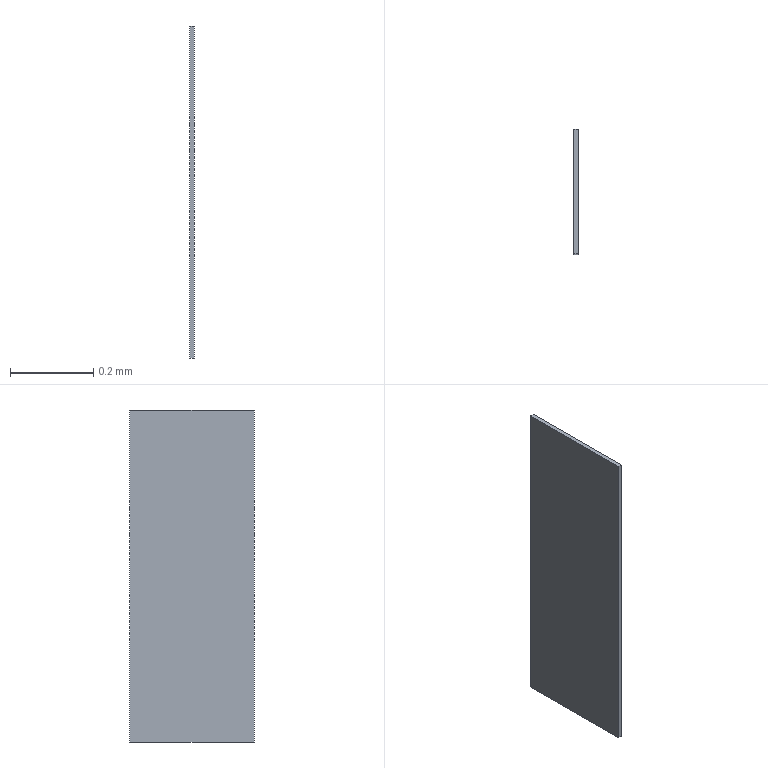Part | Creo | 1 solid | 6 faces | box 0.01 x 0.3 x 0.8 mm | volume 0.0024 mm3 | plane 6
STEP:
#1=CARTESIAN_POINT('',(0.,0.,0.));
#2=DIRECTION('',(0.,0.,1.));
#3=DIRECTION('',(1.,0.,0.));
#4=AXIS2_PLACEMENT_3D('',#1,#2,#3);
#5=CARTESIAN_POINT('',(0.12,-5.55,1.08));
#6=VERTEX_POINT('',#5);
#7=CARTESIAN_POINT('',(0.12,-5.55,1.88));
#8=VERTEX_POINT('',#7);
#9=CARTESIAN_POINT('',(0.12,-5.55,1.08));
#10=DIRECTION('',(0.,0.,1.));
#11=VECTOR('',#10,0.8);
#12=LINE('',#9,#11);
#13=EDGE_CURVE('',#6,#8,#12,.T.);
#14=ORIENTED_EDGE('',*,*,#13,.F.);
#15=CARTESIAN_POINT('',(0.12,-5.85,1.08));
#16=VERTEX_POINT('',#15);
#17=CARTESIAN_POINT('',(0.12,-5.85,1.08));
#18=DIRECTION('',(0.,1.,0.));
#19=VECTOR('',#18,0.3);
#20=LINE('',#17,#19);
#21=EDGE_CURVE('',#16,#6,#20,.T.);
#22=ORIENTED_EDGE('',*,*,#21,.F.);
#23=CARTESIAN_POINT('',(0.12,-5.85,1.88));
#24=VERTEX_POINT('',#23);
#25=CARTESIAN_POINT('',(0.12,-5.85,1.88));
#26=DIRECTION('',(0.,0.,-1.));
#27=VECTOR('',#26,0.8);
#28=LINE('',#25,#27);
#29=EDGE_CURVE('',#24,#16,#28,.T.);
#30=ORIENTED_EDGE('',*,*,#29,.F.);
#31=CARTESIAN_POINT('',(0.12,-5.55,1.88));
#32=DIRECTION('',(0.,-1.,0.));
#33=VECTOR('',#32,0.3);
#34=LINE('',#31,#33);
#35=EDGE_CURVE('',#8,#24,#34,.T.);
#36=ORIENTED_EDGE('',*,*,#35,.F.);
#37=EDGE_LOOP('',(#14,#22,#30,#36));
#38=FACE_OUTER_BOUND('',#37,.F.);
#39=CARTESIAN_POINT('',(0.12,0.,0.));
#40=DIRECTION('',(1.,0.,0.));
#41=DIRECTION('',(0.,-1.,0.));
#42=AXIS2_PLACEMENT_3D('',#39,#40,#41);
#43=PLANE('',#42);
#44=ADVANCED_FACE('',(#38),#43,.T.);
#45=CARTESIAN_POINT('',(0.11,-5.55,1.08));
#46=VERTEX_POINT('',#45);
#47=CARTESIAN_POINT('',(0.11,-5.55,1.88));
#48=VERTEX_POINT('',#47);
#49=CARTESIAN_POINT('',(0.11,-5.55,1.08));
#50=DIRECTION('',(0.,0.,1.));
#51=VECTOR('',#50,0.8);
#52=LINE('',#49,#51);
#53=EDGE_CURVE('',#46,#48,#52,.T.);
#54=ORIENTED_EDGE('',*,*,#53,.F.);
#55=CARTESIAN_POINT('',(0.11,-5.55,1.08));
#56=DIRECTION('',(1.,0.,0.));
#57=VECTOR('',#56,0.01);
#58=LINE('',#55,#57);
#59=EDGE_CURVE('',#46,#6,#58,.T.);
#60=ORIENTED_EDGE('',*,*,#59,.T.);
#61=ORIENTED_EDGE('',*,*,#13,.T.);
#62=CARTESIAN_POINT('',(0.11,-5.55,1.88));
#63=DIRECTION('',(1.,0.,0.));
#64=VECTOR('',#63,0.01);
#65=LINE('',#62,#64);
#66=EDGE_CURVE('',#48,#8,#65,.T.);
#67=ORIENTED_EDGE('',*,*,#66,.F.);
#68=EDGE_LOOP('',(#54,#60,#61,#67));
#69=FACE_OUTER_BOUND('',#68,.F.);
#70=CARTESIAN_POINT('',(0.,-5.55,1.08));
#71=DIRECTION('',(0.,1.,0.));
#72=DIRECTION('',(0.,0.,1.));
#73=AXIS2_PLACEMENT_3D('',#70,#71,#72);
#74=PLANE('',#73);
#75=ADVANCED_FACE('',(#69),#74,.T.);
#76=ORIENTED_EDGE('',*,*,#53,.T.);
#77=CARTESIAN_POINT('',(0.11,-5.85,1.88));
#78=VERTEX_POINT('',#77);
#79=CARTESIAN_POINT('',(0.11,-5.55,1.88));
#80=DIRECTION('',(0.,-1.,0.));
#81=VECTOR('',#80,0.3);
#82=LINE('',#79,#81);
#83=EDGE_CURVE('',#48,#78,#82,.T.);
#84=ORIENTED_EDGE('',*,*,#83,.T.);
#85=CARTESIAN_POINT('',(0.11,-5.85,1.08));
#86=VERTEX_POINT('',#85);
#87=CARTESIAN_POINT('',(0.11,-5.85,1.88));
#88=DIRECTION('',(0.,0.,-1.));
#89=VECTOR('',#88,0.8);
#90=LINE('',#87,#89);
#91=EDGE_CURVE('',#78,#86,#90,.T.);
#92=ORIENTED_EDGE('',*,*,#91,.T.);
#93=CARTESIAN_POINT('',(0.11,-5.85,1.08));
#94=DIRECTION('',(0.,1.,0.));
#95=VECTOR('',#94,0.3);
#96=LINE('',#93,#95);
#97=EDGE_CURVE('',#86,#46,#96,.T.);
#98=ORIENTED_EDGE('',*,*,#97,.T.);
#99=EDGE_LOOP('',(#76,#84,#92,#98));
#100=FACE_OUTER_BOUND('',#99,.F.);
#101=CARTESIAN_POINT('',(0.11,-11.395,4.186));
#102=DIRECTION('',(1.,0.,0.));
#103=DIRECTION('',(0.,1.,0.));
#104=AXIS2_PLACEMENT_3D('',#101,#102,#103);
#105=PLANE('',#104);
#106=ADVANCED_FACE('',(#100),#105,.F.);
#107=ORIENTED_EDGE('',*,*,#83,.F.);
#108=ORIENTED_EDGE('',*,*,#66,.T.);
#109=ORIENTED_EDGE('',*,*,#35,.T.);
#110=CARTESIAN_POINT('',(0.11,-5.85,1.88));
#111=DIRECTION('',(1.,0.,0.));
#112=VECTOR('',#111,0.01);
#113=LINE('',#110,#112);
#114=EDGE_CURVE('',#78,#24,#113,.T.);
#115=ORIENTED_EDGE('',*,*,#114,.F.);
#116=EDGE_LOOP('',(#107,#108,#109,#115));
#117=FACE_OUTER_BOUND('',#116,.F.);
#118=CARTESIAN_POINT('',(0.,-5.55,1.88));
#119=DIRECTION('',(0.,0.,1.));
#120=DIRECTION('',(0.,-1.,0.));
#121=AXIS2_PLACEMENT_3D('',#118,#119,#120);
#122=PLANE('',#121);
#123=ADVANCED_FACE('',(#117),#122,.T.);
#124=ORIENTED_EDGE('',*,*,#91,.F.);
#125=ORIENTED_EDGE('',*,*,#114,.T.);
#126=ORIENTED_EDGE('',*,*,#29,.T.);
#127=CARTESIAN_POINT('',(0.11,-5.85,1.08));
#128=DIRECTION('',(1.,0.,0.));
#129=VECTOR('',#128,0.01);
#130=LINE('',#127,#129);
#131=EDGE_CURVE('',#86,#16,#130,.T.);
#132=ORIENTED_EDGE('',*,*,#131,.F.);
#133=EDGE_LOOP('',(#124,#125,#126,#132));
#134=FACE_OUTER_BOUND('',#133,.F.);
#135=CARTESIAN_POINT('',(0.,-5.85,1.88));
#136=DIRECTION('',(0.,-1.,0.));
#137=DIRECTION('',(0.,0.,-1.));
#138=AXIS2_PLACEMENT_3D('',#135,#136,#137);
#139=PLANE('',#138);
#140=ADVANCED_FACE('',(#134),#139,.T.);
#141=ORIENTED_EDGE('',*,*,#97,.F.);
#142=ORIENTED_EDGE('',*,*,#131,.T.);
#143=ORIENTED_EDGE('',*,*,#21,.T.);
#144=ORIENTED_EDGE('',*,*,#59,.F.);
#145=EDGE_LOOP('',(#141,#142,#143,#144));
#146=FACE_OUTER_BOUND('',#145,.F.);
#147=CARTESIAN_POINT('',(0.,-5.85,1.08));
#148=DIRECTION('',(0.,0.,-1.));
#149=DIRECTION('',(0.,1.,0.));
#150=AXIS2_PLACEMENT_3D('',#147,#148,#149);
#151=PLANE('',#150);
#152=ADVANCED_FACE('',(#146),#151,.T.);
#153=CLOSED_SHELL('',(#44,#75,#106,#123,#140,#152));
#154=MANIFOLD_SOLID_BREP('',#153);
#155=(LENGTH_UNIT()NAMED_UNIT(*)SI_UNIT(.MILLI.,.METRE.));
#156=UNCERTAINTY_MEASURE_WITH_UNIT(LENGTH_MEASURE(0.00008544),#155,'','');
#157=(NAMED_UNIT(*)PLANE_ANGLE_UNIT()SI_UNIT($,.RADIAN.));
#158=PLANE_ANGLE_MEASURE_WITH_UNIT(PLANE_ANGLE_MEASURE(0.01745),#157);
#159=(CONVERSION_BASED_UNIT('DEGREE',#158)NAMED_UNIT(*)PLANE_ANGLE_UNIT());
#160=(NAMED_UNIT(*)SI_UNIT($,.STERADIAN.)SOLID_ANGLE_UNIT());
#161=(GEOMETRIC_REPRESENTATION_CONTEXT(3)GLOBAL_UNCERTAINTY_ASSIGNED_CONTEXT((#156))GLOBAL_UNIT_ASSIGNED_CONTEXT((#155,#159,#160))REPRESENTATION_CONTEXT('',''));
#162=ADVANCED_BREP_SHAPE_REPRESENTATION('',(#4,#154),#161);